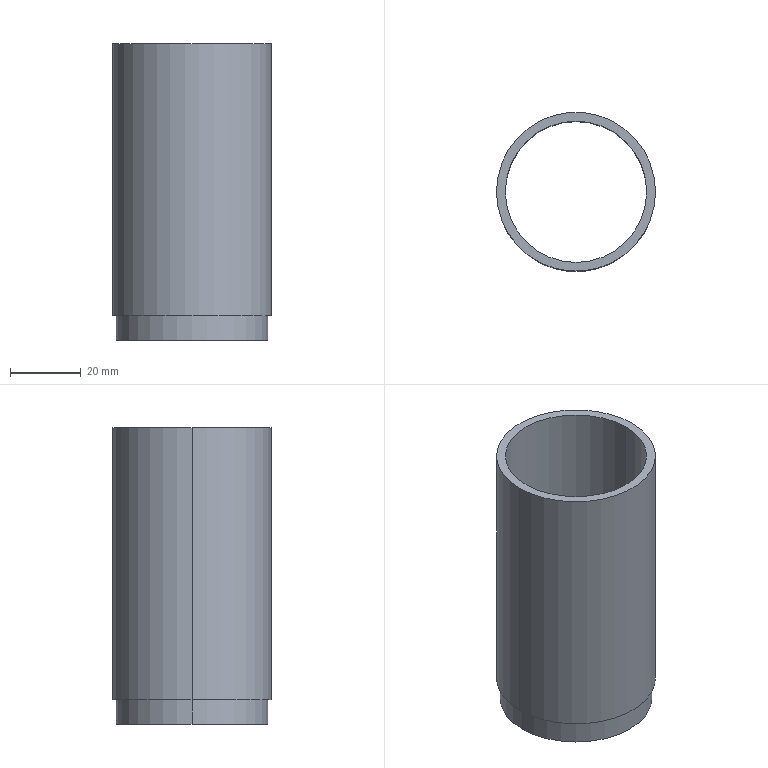Part | SolidWorks | features Extrusion 1, ICE 1 | 1 solid | 9 faces | box 45 x 45 x 84 mm | volume 27071 mm3 | cylinder 6 | plane 3 | commonest cylinder face diameters 40 x2 43 x2 45 x2
STEP:
#1=CARTESIAN_POINT('',(-21.5,0.,7.));
#2=VERTEX_POINT('',#1);
#3=CARTESIAN_POINT('',(21.5,0.,7.));
#4=VERTEX_POINT('',#3);
#5=CARTESIAN_POINT('',(0.,0.,7.));
#6=DIRECTION('',(0.,0.,-1.));
#7=DIRECTION('',(-1.,0.,0.));
#8=AXIS2_PLACEMENT_3D('',#5,#6,#7);
#9=CIRCLE('',#8,21.5);
#10=EDGE_CURVE('',#2,#4,#9,.T.);
#11=ORIENTED_EDGE('',*,*,#10,.T.);
#12=CARTESIAN_POINT('',(21.5,0.,0.));
#13=VERTEX_POINT('',#12);
#14=CARTESIAN_POINT('',(21.5,0.,7.));
#15=DIRECTION('',(0.,0.,-1.));
#16=VECTOR('',#15,1000.);
#17=LINE('',#14,#16);
#18=EDGE_CURVE('',#4,#13,#17,.T.);
#19=ORIENTED_EDGE('',*,*,#18,.T.);
#20=CARTESIAN_POINT('',(-21.5,0.,0.));
#21=VERTEX_POINT('',#20);
#22=CARTESIAN_POINT('',(0.,0.,0.));
#23=DIRECTION('',(0.,0.,-1.));
#24=DIRECTION('',(-1.,0.,0.));
#25=AXIS2_PLACEMENT_3D('',#22,#23,#24);
#26=CIRCLE('',#25,21.5);
#27=EDGE_CURVE('',#21,#13,#26,.T.);
#28=ORIENTED_EDGE('',*,*,#27,.F.);
#29=CARTESIAN_POINT('',(-21.5,0.,7.));
#30=DIRECTION('',(0.,0.,-1.));
#31=VECTOR('',#30,1000.);
#32=LINE('',#29,#31);
#33=EDGE_CURVE('',#2,#21,#32,.T.);
#34=ORIENTED_EDGE('',*,*,#33,.F.);
#35=EDGE_LOOP('',(#11,#19,#28,#34));
#36=FACE_OUTER_BOUND('',#35,.T.);
#37=CARTESIAN_POINT('',(0.,0.,7.));
#38=DIRECTION('',(0.,0.,-1.));
#39=DIRECTION('',(-1.,0.,0.));
#40=AXIS2_PLACEMENT_3D('',#37,#38,#39);
#41=CYLINDRICAL_SURFACE('',#40,21.5);
#42=ADVANCED_FACE('',(#36),#41,.T.);
#43=CARTESIAN_POINT('',(-20.,0.,84.));
#44=VERTEX_POINT('',#43);
#45=CARTESIAN_POINT('',(20.,0.,84.));
#46=VERTEX_POINT('',#45);
#47=CARTESIAN_POINT('',(0.,0.,84.));
#48=DIRECTION('',(0.,0.,1.));
#49=DIRECTION('',(1.,0.,0.));
#50=AXIS2_PLACEMENT_3D('',#47,#48,#49);
#51=CIRCLE('',#50,20.);
#52=EDGE_CURVE('',#44,#46,#51,.T.);
#53=ORIENTED_EDGE('',*,*,#52,.T.);
#54=CARTESIAN_POINT('',(20.,0.,0.));
#55=VERTEX_POINT('',#54);
#56=CARTESIAN_POINT('',(20.,0.,84.));
#57=DIRECTION('',(0.,0.,-1.));
#58=VECTOR('',#57,1000.);
#59=LINE('',#56,#58);
#60=EDGE_CURVE('',#46,#55,#59,.T.);
#61=ORIENTED_EDGE('',*,*,#60,.T.);
#62=CARTESIAN_POINT('',(-20.,0.,0.));
#63=VERTEX_POINT('',#62);
#64=CARTESIAN_POINT('',(0.,0.,0.));
#65=DIRECTION('',(0.,0.,1.));
#66=DIRECTION('',(1.,0.,0.));
#67=AXIS2_PLACEMENT_3D('',#64,#65,#66);
#68=CIRCLE('',#67,20.);
#69=EDGE_CURVE('',#63,#55,#68,.T.);
#70=ORIENTED_EDGE('',*,*,#69,.F.);
#71=CARTESIAN_POINT('',(-20.,0.,84.));
#72=DIRECTION('',(0.,0.,-1.));
#73=VECTOR('',#72,1000.);
#74=LINE('',#71,#73);
#75=EDGE_CURVE('',#44,#63,#74,.T.);
#76=ORIENTED_EDGE('',*,*,#75,.F.);
#77=EDGE_LOOP('',(#53,#61,#70,#76));
#78=FACE_OUTER_BOUND('',#77,.T.);
#79=CARTESIAN_POINT('',(0.,0.,84.));
#80=DIRECTION('',(0.,0.,-1.));
#81=DIRECTION('',(-1.,0.,0.));
#82=AXIS2_PLACEMENT_3D('',#79,#80,#81);
#83=CYLINDRICAL_SURFACE('',#82,20.);
#84=ADVANCED_FACE('',(#78),#83,.F.);
#85=CARTESIAN_POINT('',(22.5,0.,84.));
#86=VERTEX_POINT('',#85);
#87=CARTESIAN_POINT('',(-22.5,0.,84.));
#88=VERTEX_POINT('',#87);
#89=CARTESIAN_POINT('',(0.,0.,84.));
#90=DIRECTION('',(0.,0.,1.));
#91=DIRECTION('',(1.,0.,0.));
#92=AXIS2_PLACEMENT_3D('',#89,#90,#91);
#93=CIRCLE('',#92,22.5);
#94=EDGE_CURVE('',#86,#88,#93,.T.);
#95=ORIENTED_EDGE('',*,*,#94,.F.);
#96=CARTESIAN_POINT('',(22.5,0.,7.));
#97=VERTEX_POINT('',#96);
#98=CARTESIAN_POINT('',(22.5,0.,84.));
#99=DIRECTION('',(0.,0.,-1.));
#100=VECTOR('',#99,1000.);
#101=LINE('',#98,#100);
#102=EDGE_CURVE('',#86,#97,#101,.T.);
#103=ORIENTED_EDGE('',*,*,#102,.T.);
#104=CARTESIAN_POINT('',(-22.5,0.,7.));
#105=VERTEX_POINT('',#104);
#106=CARTESIAN_POINT('',(0.,0.,7.));
#107=DIRECTION('',(0.,0.,-1.));
#108=DIRECTION('',(-1.,0.,0.));
#109=AXIS2_PLACEMENT_3D('',#106,#107,#108);
#110=CIRCLE('',#109,22.5);
#111=EDGE_CURVE('',#105,#97,#110,.T.);
#112=ORIENTED_EDGE('',*,*,#111,.F.);
#113=CARTESIAN_POINT('',(-22.5,0.,84.));
#114=DIRECTION('',(0.,0.,-1.));
#115=VECTOR('',#114,1000.);
#116=LINE('',#113,#115);
#117=EDGE_CURVE('',#88,#105,#116,.T.);
#118=ORIENTED_EDGE('',*,*,#117,.F.);
#119=EDGE_LOOP('',(#95,#103,#112,#118));
#120=FACE_OUTER_BOUND('',#119,.T.);
#121=CARTESIAN_POINT('',(0.,0.,84.));
#122=DIRECTION('',(0.,0.,-1.));
#123=DIRECTION('',(-1.,0.,0.));
#124=AXIS2_PLACEMENT_3D('',#121,#122,#123);
#125=CYLINDRICAL_SURFACE('',#124,22.5);
#126=ADVANCED_FACE('',(#120),#125,.T.);
#127=ORIENTED_EDGE('',*,*,#69,.T.);
#128=CARTESIAN_POINT('',(0.,0.,0.));
#129=DIRECTION('',(0.,0.,1.));
#130=DIRECTION('',(1.,0.,0.));
#131=AXIS2_PLACEMENT_3D('',#128,#129,#130);
#132=CIRCLE('',#131,20.);
#133=EDGE_CURVE('',#55,#63,#132,.T.);
#134=ORIENTED_EDGE('',*,*,#133,.T.);
#135=EDGE_LOOP('',(#127,#134));
#136=FACE_BOUND('',#135,.T.);
#137=ORIENTED_EDGE('',*,*,#27,.T.);
#138=CARTESIAN_POINT('',(0.,0.,0.));
#139=DIRECTION('',(0.,0.,-1.));
#140=DIRECTION('',(-1.,0.,0.));
#141=AXIS2_PLACEMENT_3D('',#138,#139,#140);
#142=CIRCLE('',#141,21.5);
#143=EDGE_CURVE('',#13,#21,#142,.T.);
#144=ORIENTED_EDGE('',*,*,#143,.T.);
#145=EDGE_LOOP('',(#137,#144));
#146=FACE_OUTER_BOUND('',#145,.T.);
#147=CARTESIAN_POINT('',(0.,0.,0.));
#148=DIRECTION('',(0.,0.,1.));
#149=DIRECTION('',(1.,0.,0.));
#150=AXIS2_PLACEMENT_3D('',#147,#148,#149);
#151=PLANE('',#150);
#152=ADVANCED_FACE('',(#136,#146),#151,.F.);
#153=ORIENTED_EDGE('',*,*,#102,.F.);
#154=CARTESIAN_POINT('',(0.,0.,84.));
#155=DIRECTION('',(0.,0.,1.));
#156=DIRECTION('',(1.,0.,0.));
#157=AXIS2_PLACEMENT_3D('',#154,#155,#156);
#158=CIRCLE('',#157,22.5);
#159=EDGE_CURVE('',#88,#86,#158,.T.);
#160=ORIENTED_EDGE('',*,*,#159,.F.);
#161=ORIENTED_EDGE('',*,*,#117,.T.);
#162=CARTESIAN_POINT('',(0.,0.,7.));
#163=DIRECTION('',(0.,0.,-1.));
#164=DIRECTION('',(-1.,0.,0.));
#165=AXIS2_PLACEMENT_3D('',#162,#163,#164);
#166=CIRCLE('',#165,22.5);
#167=EDGE_CURVE('',#97,#105,#166,.T.);
#168=ORIENTED_EDGE('',*,*,#167,.F.);
#169=EDGE_LOOP('',(#153,#160,#161,#168));
#170=FACE_OUTER_BOUND('',#169,.T.);
#171=CARTESIAN_POINT('',(0.,0.,84.));
#172=DIRECTION('',(0.,0.,-1.));
#173=DIRECTION('',(-1.,0.,0.));
#174=AXIS2_PLACEMENT_3D('',#171,#172,#173);
#175=CYLINDRICAL_SURFACE('',#174,22.5);
#176=ADVANCED_FACE('',(#170),#175,.T.);
#177=ORIENTED_EDGE('',*,*,#159,.T.);
#178=ORIENTED_EDGE('',*,*,#94,.T.);
#179=EDGE_LOOP('',(#177,#178));
#180=FACE_OUTER_BOUND('',#179,.T.);
#181=ORIENTED_EDGE('',*,*,#52,.F.);
#182=CARTESIAN_POINT('',(0.,0.,84.));
#183=DIRECTION('',(0.,0.,1.));
#184=DIRECTION('',(1.,0.,0.));
#185=AXIS2_PLACEMENT_3D('',#182,#183,#184);
#186=CIRCLE('',#185,20.);
#187=EDGE_CURVE('',#46,#44,#186,.T.);
#188=ORIENTED_EDGE('',*,*,#187,.F.);
#189=EDGE_LOOP('',(#181,#188));
#190=FACE_BOUND('',#189,.T.);
#191=CARTESIAN_POINT('',(0.,0.,84.));
#192=DIRECTION('',(0.,0.,1.));
#193=DIRECTION('',(1.,0.,0.));
#194=AXIS2_PLACEMENT_3D('',#191,#192,#193);
#195=PLANE('',#194);
#196=ADVANCED_FACE('',(#180,#190),#195,.T.);
#197=ORIENTED_EDGE('',*,*,#60,.F.);
#198=ORIENTED_EDGE('',*,*,#187,.T.);
#199=ORIENTED_EDGE('',*,*,#75,.T.);
#200=ORIENTED_EDGE('',*,*,#133,.F.);
#201=EDGE_LOOP('',(#197,#198,#199,#200));
#202=FACE_OUTER_BOUND('',#201,.T.);
#203=CARTESIAN_POINT('',(0.,0.,84.));
#204=DIRECTION('',(0.,0.,-1.));
#205=DIRECTION('',(-1.,0.,0.));
#206=AXIS2_PLACEMENT_3D('',#203,#204,#205);
#207=CYLINDRICAL_SURFACE('',#206,20.);
#208=ADVANCED_FACE('',(#202),#207,.F.);
#209=ORIENTED_EDGE('',*,*,#10,.F.);
#210=CARTESIAN_POINT('',(0.,0.,7.));
#211=DIRECTION('',(0.,0.,-1.));
#212=DIRECTION('',(-1.,0.,0.));
#213=AXIS2_PLACEMENT_3D('',#210,#211,#212);
#214=CIRCLE('',#213,21.5);
#215=EDGE_CURVE('',#4,#2,#214,.T.);
#216=ORIENTED_EDGE('',*,*,#215,.F.);
#217=EDGE_LOOP('',(#209,#216));
#218=FACE_BOUND('',#217,.T.);
#219=ORIENTED_EDGE('',*,*,#111,.T.);
#220=ORIENTED_EDGE('',*,*,#167,.T.);
#221=EDGE_LOOP('',(#219,#220));
#222=FACE_OUTER_BOUND('',#221,.T.);
#223=CARTESIAN_POINT('',(0.,0.,7.));
#224=DIRECTION('',(0.,0.,-1.));
#225=DIRECTION('',(-1.,0.,0.));
#226=AXIS2_PLACEMENT_3D('',#223,#224,#225);
#227=PLANE('',#226);
#228=ADVANCED_FACE('',(#218,#222),#227,.T.);
#229=ORIENTED_EDGE('',*,*,#18,.F.);
#230=ORIENTED_EDGE('',*,*,#215,.T.);
#231=ORIENTED_EDGE('',*,*,#33,.T.);
#232=ORIENTED_EDGE('',*,*,#143,.F.);
#233=EDGE_LOOP('',(#229,#230,#231,#232));
#234=FACE_OUTER_BOUND('',#233,.T.);
#235=CARTESIAN_POINT('',(0.,0.,7.));
#236=DIRECTION('',(0.,0.,-1.));
#237=DIRECTION('',(-1.,0.,0.));
#238=AXIS2_PLACEMENT_3D('',#235,#236,#237);
#239=CYLINDRICAL_SURFACE('',#238,21.5);
#240=ADVANCED_FACE('',(#234),#239,.T.);
#241=CLOSED_SHELL('',(#42,#84,#126,#152,#176,#196,#208,#228,#240));
#242=MANIFOLD_SOLID_BREP('',#241);
#243=CARTESIAN_POINT('',(0.,0.,0.));
#244=DIRECTION('',(0.,0.,1.));
#245=DIRECTION('',(1.,0.,0.));
#246=AXIS2_PLACEMENT_3D('',#243,#244,#245);
#247=(LENGTH_UNIT()NAMED_UNIT(*)SI_UNIT(.MILLI.,.METRE.));
#248=UNCERTAINTY_MEASURE_WITH_UNIT(LENGTH_MEASURE(0.00001),#247,'','');
#249=(NAMED_UNIT(*)PLANE_ANGLE_UNIT()SI_UNIT($,.RADIAN.));
#250=(NAMED_UNIT(*)SI_UNIT($,.STERADIAN.)SOLID_ANGLE_UNIT());
#251=(GEOMETRIC_REPRESENTATION_CONTEXT(3)GLOBAL_UNCERTAINTY_ASSIGNED_CONTEXT((#248))GLOBAL_UNIT_ASSIGNED_CONTEXT((#247,#249,#250))REPRESENTATION_CONTEXT('',''));
#252=ADVANCED_BREP_SHAPE_REPRESENTATION('',(#242,#246),#251);